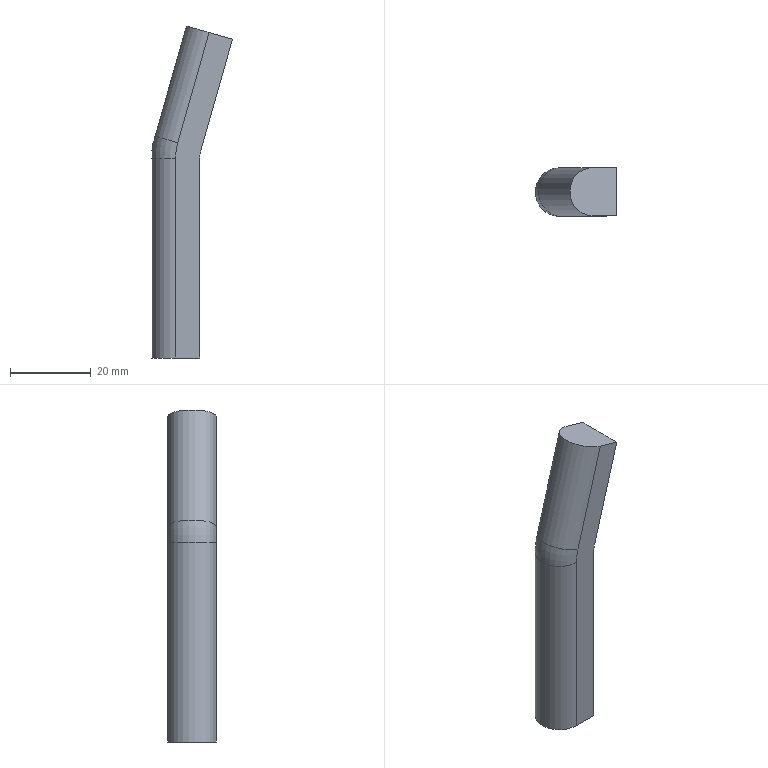Part | NX | features solid 2 | 1 solid | 10 faces | box 20.071 x 12 x 82.272 mm | volume 10491 mm3 | plane 6 | cylinder 3 | torus 1 | commonest cylinder face diameters 12 x2 16 x1
STEP:
#1=CARTESIAN_POINT('',(821.,357.,54.523));
#2=VERTEX_POINT('',#1);
#3=CARTESIAN_POINT('',(821.,345.,54.523));
#4=VERTEX_POINT('',#3);
#5=CARTESIAN_POINT('',(821.,351.,54.523));
#6=DIRECTION('',(0.,0.,1.));
#7=DIRECTION('',(-1.,0.,0.));
#8=AXIS2_PLACEMENT_3D('',#5,#6,#7);
#9=CIRCLE('',#8,6.);
#10=EDGE_CURVE('',#2,#4,#9,.T.);
#11=ORIENTED_EDGE('',*,*,#10,.T.);
#12=CARTESIAN_POINT('',(821.535,345.,58.357));
#13=VERTEX_POINT('',#12);
#14=CARTESIAN_POINT('',(835.,345.,54.523));
#15=DIRECTION('',(0.,1.,0.));
#16=DIRECTION('',(0.,0.,-1.));
#17=AXIS2_PLACEMENT_3D('',#14,#15,#16);
#18=CIRCLE('',#17,14.);
#19=EDGE_CURVE('',#4,#13,#18,.T.);
#20=ORIENTED_EDGE('',*,*,#19,.T.);
#21=CARTESIAN_POINT('',(821.535,357.,58.357));
#22=VERTEX_POINT('',#21);
#23=CARTESIAN_POINT('',(821.535,351.,58.357));
#24=DIRECTION('',(0.2738,0.,0.9618));
#25=DIRECTION('',(-0.9618,0.,0.2738));
#26=AXIS2_PLACEMENT_3D('',#23,#24,#25);
#27=CIRCLE('',#26,6.);
#28=EDGE_CURVE('',#22,#13,#27,.T.);
#29=ORIENTED_EDGE('',*,*,#28,.F.);
#30=CARTESIAN_POINT('',(835.,357.,54.523));
#31=DIRECTION('',(0.,1.,0.));
#32=DIRECTION('',(0.,0.,-1.));
#33=AXIS2_PLACEMENT_3D('',#30,#31,#32);
#34=CIRCLE('',#33,14.);
#35=EDGE_CURVE('',#2,#22,#34,.T.);
#36=ORIENTED_EDGE('',*,*,#35,.F.);
#37=EDGE_LOOP('',(#11,#20,#29,#36));
#38=FACE_BOUND('',#37,.T.);
#39=CARTESIAN_POINT('',(835.,351.,54.523));
#40=DIRECTION('',(0.,1.,0.));
#41=DIRECTION('',(0.,0.,-1.));
#42=AXIS2_PLACEMENT_3D('',#39,#40,#41);
#43=TOROIDAL_SURFACE('',#42,14.,6.);
#44=ADVANCED_FACE('',(#38),#43,.T.);
#45=CARTESIAN_POINT('',(821.,345.,5.));
#46=VERTEX_POINT('',#45);
#47=CARTESIAN_POINT('',(821.,345.,79.523));
#48=DIRECTION('',(0.,0.,-1.));
#49=VECTOR('',#48,1000.);
#50=LINE('',#47,#49);
#51=EDGE_CURVE('',#4,#46,#50,.T.);
#52=ORIENTED_EDGE('',*,*,#51,.F.);
#53=ORIENTED_EDGE('',*,*,#10,.F.);
#54=CARTESIAN_POINT('',(821.,357.,5.));
#55=VERTEX_POINT('',#54);
#56=CARTESIAN_POINT('',(821.,357.,79.523));
#57=DIRECTION('',(0.,0.,-1.));
#58=VECTOR('',#57,1000.);
#59=LINE('',#56,#58);
#60=EDGE_CURVE('',#2,#55,#59,.T.);
#61=ORIENTED_EDGE('',*,*,#60,.T.);
#62=CARTESIAN_POINT('',(821.,351.,5.));
#63=DIRECTION('',(0.,0.,1.));
#64=DIRECTION('',(1.,0.,0.));
#65=AXIS2_PLACEMENT_3D('',#62,#63,#64);
#66=CIRCLE('',#65,6.);
#67=EDGE_CURVE('',#55,#46,#66,.T.);
#68=ORIENTED_EDGE('',*,*,#67,.T.);
#69=EDGE_LOOP('',(#52,#53,#61,#68));
#70=FACE_BOUND('',#69,.T.);
#71=CARTESIAN_POINT('',(821.,351.,79.523));
#72=DIRECTION('',(0.,0.,-1.));
#73=DIRECTION('',(1.,0.,0.));
#74=AXIS2_PLACEMENT_3D('',#71,#72,#73);
#75=CYLINDRICAL_SURFACE('',#74,6.);
#76=ADVANCED_FACE('',(#70),#75,.T.);
#77=CARTESIAN_POINT('',(827.,357.,54.523));
#78=VERTEX_POINT('',#77);
#79=CARTESIAN_POINT('',(827.,357.,5.));
#80=VERTEX_POINT('',#79);
#81=CARTESIAN_POINT('',(827.,357.,89.523));
#82=DIRECTION('',(0.,0.,-1.));
#83=VECTOR('',#82,1000.);
#84=LINE('',#81,#83);
#85=EDGE_CURVE('',#78,#80,#84,.T.);
#86=ORIENTED_EDGE('',*,*,#85,.F.);
#87=CARTESIAN_POINT('',(827.,345.,54.523));
#88=VERTEX_POINT('',#87);
#89=CARTESIAN_POINT('',(827.,381.,54.523));
#90=DIRECTION('',(0.,1.,0.));
#91=VECTOR('',#90,1000.);
#92=LINE('',#89,#91);
#93=EDGE_CURVE('',#88,#78,#92,.T.);
#94=ORIENTED_EDGE('',*,*,#93,.F.);
#95=CARTESIAN_POINT('',(827.,345.,5.));
#96=VERTEX_POINT('',#95);
#97=CARTESIAN_POINT('',(827.,345.,89.523));
#98=DIRECTION('',(0.,0.,-1.));
#99=VECTOR('',#98,1000.);
#100=LINE('',#97,#99);
#101=EDGE_CURVE('',#88,#96,#100,.T.);
#102=ORIENTED_EDGE('',*,*,#101,.T.);
#103=CARTESIAN_POINT('',(827.,381.,5.));
#104=DIRECTION('',(0.,1.,0.));
#105=VECTOR('',#104,1000.);
#106=LINE('',#103,#105);
#107=EDGE_CURVE('',#96,#80,#106,.T.);
#108=ORIENTED_EDGE('',*,*,#107,.T.);
#109=EDGE_LOOP('',(#86,#94,#102,#108));
#110=FACE_BOUND('',#109,.T.);
#111=CARTESIAN_POINT('',(827.,381.,89.523));
#112=DIRECTION('',(-1.,0.,0.));
#113=DIRECTION('',(0.,-1.,0.));
#114=AXIS2_PLACEMENT_3D('',#111,#112,#113);
#115=PLANE('',#114);
#116=ADVANCED_FACE('',(#110),#115,.F.);
#117=ORIENTED_EDGE('',*,*,#107,.F.);
#118=CARTESIAN_POINT('',(919.,345.,5.));
#119=DIRECTION('',(1.,0.,0.));
#120=VECTOR('',#119,1000.);
#121=LINE('',#118,#120);
#122=EDGE_CURVE('',#46,#96,#121,.T.);
#123=ORIENTED_EDGE('',*,*,#122,.F.);
#124=ORIENTED_EDGE('',*,*,#67,.F.);
#125=CARTESIAN_POINT('',(919.,357.,5.));
#126=DIRECTION('',(1.,0.,0.));
#127=VECTOR('',#126,1000.);
#128=LINE('',#125,#127);
#129=EDGE_CURVE('',#55,#80,#128,.T.);
#130=ORIENTED_EDGE('',*,*,#129,.T.);
#131=EDGE_LOOP('',(#117,#123,#124,#130));
#132=FACE_BOUND('',#131,.T.);
#133=CARTESIAN_POINT('',(852.,324.,5.));
#134=DIRECTION('',(0.,0.,1.));
#135=DIRECTION('',(0.,1.,0.));
#136=AXIS2_PLACEMENT_3D('',#133,#134,#135);
#137=PLANE('',#136);
#138=ADVANCED_FACE('',(#132),#137,.F.);
#139=ORIENTED_EDGE('',*,*,#101,.F.);
#140=CARTESIAN_POINT('',(827.306,345.,56.714));
#141=VERTEX_POINT('',#140);
#142=CARTESIAN_POINT('',(835.,345.,54.523));
#143=DIRECTION('',(0.,1.,0.));
#144=DIRECTION('',(0.,0.,-1.));
#145=AXIS2_PLACEMENT_3D('',#142,#143,#144);
#146=CIRCLE('',#145,8.);
#147=EDGE_CURVE('',#88,#141,#146,.T.);
#148=ORIENTED_EDGE('',*,*,#147,.T.);
#149=CARTESIAN_POINT('',(835.071,345.,83.986));
#150=VERTEX_POINT('',#149);
#151=CARTESIAN_POINT('',(827.306,345.,56.714));
#152=DIRECTION('',(0.2738,0.,0.9618));
#153=VECTOR('',#152,1000.);
#154=LINE('',#151,#153);
#155=EDGE_CURVE('',#141,#150,#154,.T.);
#156=ORIENTED_EDGE('',*,*,#155,.T.);
#157=CARTESIAN_POINT('',(829.3,345.,85.629));
#158=VERTEX_POINT('',#157);
#159=CARTESIAN_POINT('',(836.81,345.,83.491));
#160=DIRECTION('',(0.9618,0.,-0.2738));
#161=VECTOR('',#160,1000.);
#162=LINE('',#159,#161);
#163=EDGE_CURVE('',#158,#150,#162,.T.);
#164=ORIENTED_EDGE('',*,*,#163,.F.);
#165=CARTESIAN_POINT('',(821.535,345.,58.357));
#166=DIRECTION('',(0.2738,0.,0.9618));
#167=VECTOR('',#166,1000.);
#168=LINE('',#165,#167);
#169=EDGE_CURVE('',#13,#158,#168,.T.);
#170=ORIENTED_EDGE('',*,*,#169,.F.);
#171=ORIENTED_EDGE('',*,*,#19,.F.);
#172=ORIENTED_EDGE('',*,*,#51,.T.);
#173=ORIENTED_EDGE('',*,*,#122,.T.);
#174=EDGE_LOOP('',(#139,#148,#156,#164,#170,#171,#172,#173));
#175=FACE_BOUND('',#174,.T.);
#176=CARTESIAN_POINT('',(919.,345.,89.523));
#177=DIRECTION('',(0.,1.,0.));
#178=DIRECTION('',(-1.,0.,0.));
#179=AXIS2_PLACEMENT_3D('',#176,#177,#178);
#180=PLANE('',#179);
#181=ADVANCED_FACE('',(#175),#180,.F.);
#182=CARTESIAN_POINT('',(829.3,357.,85.629));
#183=VERTEX_POINT('',#182);
#184=CARTESIAN_POINT('',(821.535,357.,58.357));
#185=DIRECTION('',(0.2738,0.,0.9618));
#186=VECTOR('',#185,1000.);
#187=LINE('',#184,#186);
#188=EDGE_CURVE('',#22,#183,#187,.T.);
#189=ORIENTED_EDGE('',*,*,#188,.T.);
#190=CARTESIAN_POINT('',(835.071,357.,83.986));
#191=VERTEX_POINT('',#190);
#192=CARTESIAN_POINT('',(836.81,357.,83.491));
#193=DIRECTION('',(0.9618,0.,-0.2738));
#194=VECTOR('',#193,1000.);
#195=LINE('',#192,#194);
#196=EDGE_CURVE('',#183,#191,#195,.T.);
#197=ORIENTED_EDGE('',*,*,#196,.T.);
#198=CARTESIAN_POINT('',(827.306,357.,56.714));
#199=VERTEX_POINT('',#198);
#200=CARTESIAN_POINT('',(827.306,357.,56.714));
#201=DIRECTION('',(0.2738,0.,0.9618));
#202=VECTOR('',#201,1000.);
#203=LINE('',#200,#202);
#204=EDGE_CURVE('',#199,#191,#203,.T.);
#205=ORIENTED_EDGE('',*,*,#204,.F.);
#206=CARTESIAN_POINT('',(835.,357.,54.523));
#207=DIRECTION('',(0.,1.,0.));
#208=DIRECTION('',(0.,0.,-1.));
#209=AXIS2_PLACEMENT_3D('',#206,#207,#208);
#210=CIRCLE('',#209,8.);
#211=EDGE_CURVE('',#78,#199,#210,.T.);
#212=ORIENTED_EDGE('',*,*,#211,.F.);
#213=ORIENTED_EDGE('',*,*,#85,.T.);
#214=ORIENTED_EDGE('',*,*,#129,.F.);
#215=ORIENTED_EDGE('',*,*,#60,.F.);
#216=ORIENTED_EDGE('',*,*,#35,.T.);
#217=EDGE_LOOP('',(#189,#197,#205,#212,#213,#214,#215,#216));
#218=FACE_BOUND('',#217,.T.);
#219=CARTESIAN_POINT('',(919.,357.,89.523));
#220=DIRECTION('',(0.,1.,0.));
#221=DIRECTION('',(-1.,0.,0.));
#222=AXIS2_PLACEMENT_3D('',#219,#220,#221);
#223=PLANE('',#222);
#224=ADVANCED_FACE('',(#218),#223,.T.);
#225=CARTESIAN_POINT('',(829.3,351.,85.629));
#226=DIRECTION('',(-0.2738,0.,-0.9618));
#227=DIRECTION('',(-0.9618,0.,0.2738));
#228=AXIS2_PLACEMENT_3D('',#225,#226,#227);
#229=CIRCLE('',#228,6.);
#230=EDGE_CURVE('',#183,#158,#229,.F.);
#231=ORIENTED_EDGE('',*,*,#230,.T.);
#232=ORIENTED_EDGE('',*,*,#163,.T.);
#233=CARTESIAN_POINT('',(835.071,381.,83.986));
#234=DIRECTION('',(0.,1.,0.));
#235=VECTOR('',#234,1000.);
#236=LINE('',#233,#235);
#237=EDGE_CURVE('',#150,#191,#236,.T.);
#238=ORIENTED_EDGE('',*,*,#237,.T.);
#239=ORIENTED_EDGE('',*,*,#196,.F.);
#240=EDGE_LOOP('',(#231,#232,#238,#239));
#241=FACE_BOUND('',#240,.T.);
#242=CARTESIAN_POINT('',(836.81,410.75,83.491));
#243=DIRECTION('',(0.2738,0.,0.9618));
#244=DIRECTION('',(-0.9618,0.,0.2738));
#245=AXIS2_PLACEMENT_3D('',#242,#243,#244);
#246=PLANE('',#245);
#247=ADVANCED_FACE('',(#241),#246,.T.);
#248=ORIENTED_EDGE('',*,*,#230,.F.);
#249=ORIENTED_EDGE('',*,*,#188,.F.);
#250=ORIENTED_EDGE('',*,*,#28,.T.);
#251=ORIENTED_EDGE('',*,*,#169,.T.);
#252=EDGE_LOOP('',(#248,#249,#250,#251));
#253=FACE_BOUND('',#252,.T.);
#254=CARTESIAN_POINT('',(821.535,351.,58.357));
#255=DIRECTION('',(0.2738,0.,0.9618));
#256=DIRECTION('',(-0.9618,0.,0.2738));
#257=AXIS2_PLACEMENT_3D('',#254,#255,#256);
#258=CYLINDRICAL_SURFACE('',#257,6.);
#259=ADVANCED_FACE('',(#253),#258,.T.);
#260=CARTESIAN_POINT('',(827.306,381.,56.714));
#261=DIRECTION('',(0.,1.,0.));
#262=VECTOR('',#261,1000.);
#263=LINE('',#260,#262);
#264=EDGE_CURVE('',#141,#199,#263,.T.);
#265=ORIENTED_EDGE('',*,*,#264,.T.);
#266=ORIENTED_EDGE('',*,*,#204,.T.);
#267=ORIENTED_EDGE('',*,*,#237,.F.);
#268=ORIENTED_EDGE('',*,*,#155,.F.);
#269=EDGE_LOOP('',(#265,#266,#267,#268));
#270=FACE_BOUND('',#269,.T.);
#271=CARTESIAN_POINT('',(827.306,381.,56.714));
#272=DIRECTION('',(0.9618,0.,-0.2738));
#273=DIRECTION('',(0.2738,0.,0.9618));
#274=AXIS2_PLACEMENT_3D('',#271,#272,#273);
#275=PLANE('',#274);
#276=ADVANCED_FACE('',(#270),#275,.T.);
#277=ORIENTED_EDGE('',*,*,#93,.T.);
#278=ORIENTED_EDGE('',*,*,#211,.T.);
#279=ORIENTED_EDGE('',*,*,#264,.F.);
#280=ORIENTED_EDGE('',*,*,#147,.F.);
#281=EDGE_LOOP('',(#277,#278,#279,#280));
#282=FACE_BOUND('',#281,.T.);
#283=CARTESIAN_POINT('',(835.,396.,54.523));
#284=DIRECTION('',(0.,1.,0.));
#285=DIRECTION('',(0.,0.,-1.));
#286=AXIS2_PLACEMENT_3D('',#283,#284,#285);
#287=CYLINDRICAL_SURFACE('',#286,8.);
#288=ADVANCED_FACE('',(#282),#287,.F.);
#289=CLOSED_SHELL('',(#44,#76,#116,#138,#181,#224,#247,#259,#276,#288));
#290=MANIFOLD_SOLID_BREP('',#289);
#291=(LENGTH_UNIT()NAMED_UNIT(*)SI_UNIT(.MILLI.,.METRE.));
#292=UNCERTAINTY_MEASURE_WITH_UNIT(LENGTH_MEASURE(0.00001),#291,'','');
#293=(NAMED_UNIT(*)PLANE_ANGLE_UNIT()SI_UNIT($,.RADIAN.));
#294=(NAMED_UNIT(*)SI_UNIT($,.STERADIAN.)SOLID_ANGLE_UNIT());
#295=(GEOMETRIC_REPRESENTATION_CONTEXT(3)GLOBAL_UNCERTAINTY_ASSIGNED_CONTEXT((#292))GLOBAL_UNIT_ASSIGNED_CONTEXT((#291,#293,#294))REPRESENTATION_CONTEXT('',''));
#296=ADVANCED_BREP_SHAPE_REPRESENTATION('',(#290),#295);